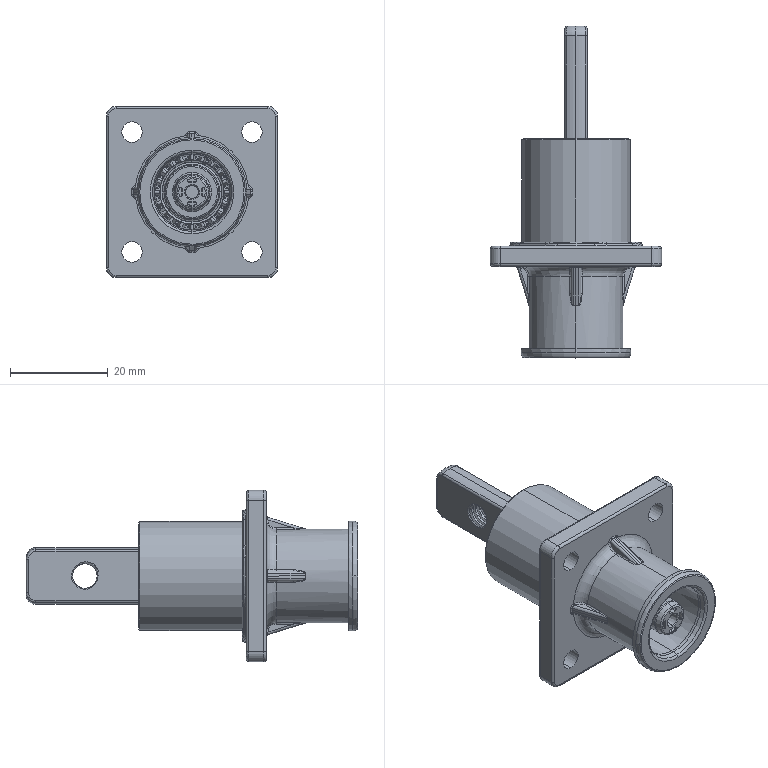Part | NX | features BREP 1 | 1 solid | 1147 faces | box 35 x 67.8 x 35 mm | volume 14088 mm3 | plane 490 | cylinder 271 | torus 182 | cone 135 | spline 69 | commonest cylinder face diameters 0.4 x86 0.6 x30 1 x22 0.7 x20 4.2 x10 5 x10